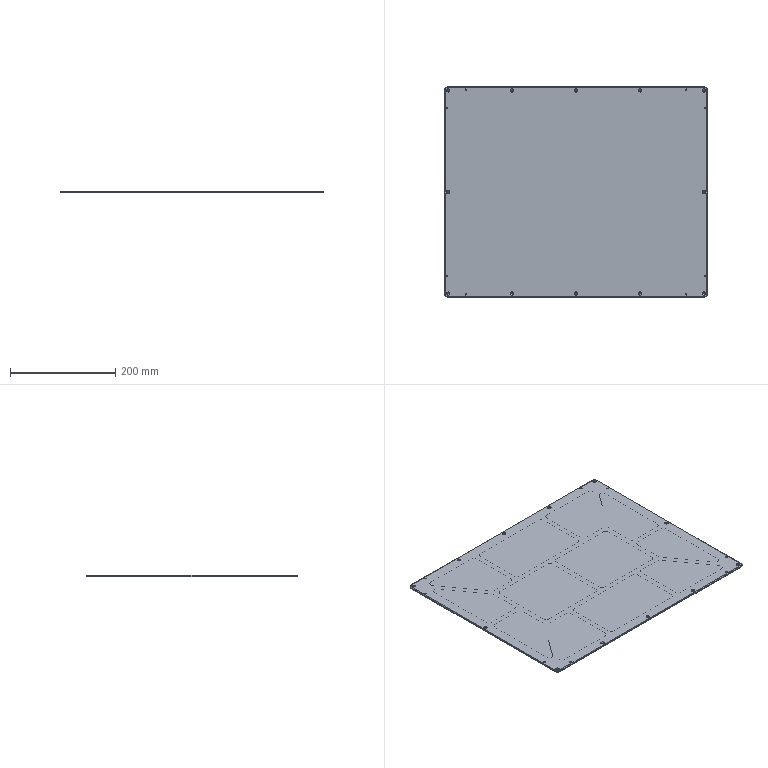NC program | Mastercam | posted with a generic post | part box 500 x 400 x 3 mm
Lines 1 to 214 of 11256:
%
:0001()
(MATERIAL - ALUMINUM MM - 2024)
(T9|10 FEM |H9|XY STOCK TO LEAVE - .15|Z STOCK TO LEAVE - .03)
(T10|10 FEM |H10|XY STOCK TO LEAVE - 0.|Z STOCK TO LEAVE - .03)
(T18|8 BNOS |H18)
(T5|4 CHM |H5)
(T8|8 FEM |H8|XY STOCK TO LEAVE - .1|Z STOCK TO LEAVE - 0.)
N100 G21
N102 G0 G17 G40 G80 G90 G94 G98
N104 G0 G28 G91 Z0.
N106 G0 G28 X0. Y0.
(10 FEM |TOOL - 9|DIA. OFF. - 9|LEN. - 9|TOOL DIA. - 10.)
N108 T9 M6
N110 G0 G54 G90 X253.177 Y-204.042 C0. B0. S10000 M3
N112 G43 H9 Z50.
N114 Z1.
N116 G1 Z0. F600.
N118 X252.57 Y-203.248 F5000.
N120 G3 X251.775 Y-202.855 I-.795 J-.607
N122 X251.168 Y-203.061 J-1.
N124 G1 X250.49 Y-203.537
N126 X249.776 Y-203.956 Z-.001
N128 X249.029 Y-204.316
N130 X248.256 Y-204.614
N132 X247.461 Y-204.847
N134 X246.65 Y-205.015 Z-.002
N136 X245.828 Y-205.116
N138 X245. Y-205.15
N140 X-245. Z-.136
N142 G2 X-255.15 Y-195. Z-.141 J10.15
N144 G1 Y195. Z-.247
N146 G2 X-245. Y205.15 Z-.252 I10.15
N148 G1 X245. Z-.386
N150 G2 X255.15 Y195. Z-.391 J-10.15
N152 G1 Y-195. Z-.497
N154 X255.115 Y-195.846
N156 X255.009 Y-196.686 Z-.498
N158 X254.834 Y-197.514
N160 X254.59 Y-198.324
N162 X254.28 Y-199.112
N164 X253.905 Y-199.871 Z-.499
N166 X253.468 Y-200.596
N168 X252.972 Y-201.282
N170 X252.421 Y-201.925
N172 X251.818 Y-202.519 Z-.5
N174 X251.168 Y-203.061
N176 X250.49 Y-203.537
N178 X249.776 Y-203.956
N180 X249.029 Y-204.316 Z-.501
N182 X248.256 Y-204.614
N184 X247.461 Y-204.847
N186 X246.65 Y-205.015
N188 X245.828 Y-205.116 Z-.502
N190 X245. Y-205.15
N192 X-245. Z-.636
N194 G2 X-255.15 Y-195. Z-.641 J10.15
N196 G1 Y195. Z-.747
N198 G2 X-245. Y205.15 Z-.752 I10.15
N200 G1 X245. Z-.886
N202 G2 X255.15 Y195. Z-.891 J-10.15
N204 G1 Y-195. Z-.997
N206 X255.115 Y-195.846
N208 X255.009 Y-196.686 Z-.998
N210 X254.834 Y-197.514
N212 X254.59 Y-198.324
N214 X254.28 Y-199.112
N216 X253.905 Y-199.871 Z-.999
N218 X253.468 Y-200.596
N220 X252.972 Y-201.282
N222 X252.421 Y-201.925
N224 X251.818 Y-202.519 Z-1.
N226 X251.168 Y-203.061
N228 X250.49 Y-203.537
N230 X249.776 Y-203.956
N232 X249.029 Y-204.316 Z-1.001
N234 X248.256 Y-204.614
N236 X247.461 Y-204.847
N238 X246.65 Y-205.015 Z-1.002
N240 X245.828 Y-205.116
N242 X245. Y-205.15
N244 X-245. Z-1.136
N246 G2 X-255.15 Y-195. Z-1.141 J10.15
N248 G1 Y195. Z-1.247
N250 G2 X-245. Y205.15 Z-1.252 I10.15
N252 G1 X245. Z-1.386
N254 G2 X255.15 Y195. Z-1.391 J-10.15
N256 G1 Y-195. Z-1.497
N258 X255.115 Y-195.846
N260 X255.009 Y-196.686 Z-1.498
N262 X254.834 Y-197.514
N264 X254.59 Y-198.324
N266 X254.28 Y-199.112
N268 X253.905 Y-199.871 Z-1.499
N270 X253.468 Y-200.596
N272 X252.972 Y-201.282
N274 X252.421 Y-201.925
N276 X251.818 Y-202.519 Z-1.5
N278 X251.168 Y-203.061
N280 X250.49 Y-203.537
N282 X249.776 Y-203.956
N284 X249.029 Y-204.316 Z-1.501
N286 X248.256 Y-204.614
N288 X247.461 Y-204.847
N290 X246.65 Y-205.015 Z-1.502
N292 X245.828 Y-205.116
N294 X245. Y-205.15
N296 X-245. Z-1.636
N298 G2 X-255.15 Y-195. Z-1.641 J10.15
N300 G1 Y195. Z-1.747
N302 G2 X-245. Y205.15 Z-1.752 I10.15
N304 G1 X245. Z-1.886
N306 G2 X255.15 Y195. Z-1.891 J-10.15
N308 G1 Y-195. Z-1.997
N310 X255.115 Y-195.846
N312 X255.009 Y-196.686 Z-1.998
N314 X254.834 Y-197.514
N316 X254.59 Y-198.324
N318 X254.28 Y-199.112
N320 X253.905 Y-199.871 Z-1.999
N322 X253.468 Y-200.596
N324 X252.972 Y-201.282
N326 X252.421 Y-201.925
N328 X251.818 Y-202.519 Z-2.
N330 X251.168 Y-203.061
N332 X250.49 Y-203.537
N334 X249.776 Y-203.956 Z-2.001
N336 X249.029 Y-204.316
N338 X248.256 Y-204.614
N340 X247.461 Y-204.847
N342 X246.65 Y-205.015 Z-2.002
N344 X245.828 Y-205.116
N346 X245. Y-205.15
N348 X-245. Z-2.136
N350 G2 X-255.15 Y-195. Z-2.141 J10.15
N352 G1 Y195. Z-2.247
N354 G2 X-245. Y205.15 Z-2.252 I10.15
N356 G1 X245. Z-2.386
N358 G2 X255.15 Y195. Z-2.391 J-10.15
N360 G1 Y-195. Z-2.497
N362 X255.115 Y-195.846
N364 X255.009 Y-196.686 Z-2.498
N366 X254.834 Y-197.514
N368 X254.59 Y-198.324
N370 X254.28 Y-199.112
N372 X253.905 Y-199.871 Z-2.499
N374 X253.468 Y-200.596
N376 X252.972 Y-201.282
N378 X252.421 Y-201.925
N380 X251.818 Y-202.519 Z-2.5
N382 X251.168 Y-203.061
N384 X250.49 Y-203.537
N386 X249.776 Y-203.956 Z-2.501
N388 X249.029 Y-204.316
N390 X248.256 Y-204.614
N392 X247.461 Y-204.847
N394 X246.65 Y-205.015 Z-2.502
N396 X245.828 Y-205.116
N398 X245. Y-205.15
N400 X-245. Z-2.636
N402 G2 X-255.15 Y-195. Z-2.641 J10.15
N404 G1 Y195. Z-2.747
N406 G2 X-245. Y205.15 Z-2.752 I10.15
N408 G1 X245. Z-2.886
N410 G2 X255.15 Y195. Z-2.891 J-10.15
N412 G1 Y-94.888 Z-2.97
N414 Y-195.
N416 G2 X251.168 Y-203.061 I-10.15
N418 X245. Y-205.15 I-6.168 J8.061
N420 G1 X-245.
N422 G2 X-255.15 Y-195. J10.15
N424 G1 Y195.
N426 G2 X-245. Y205.15 I10.15
N428 G1 X245.
N430 G2 X255.15 Y195. J-10.15
N432 G1 Y-95.388
N434 G3 X256.15 Y-96.388 I1.
N436 G1 X257.15
N438 G0 Z50.
N440 M5
N442 G0 G28 G91 Z0.
N444 G28
N446 M01
N448 G0 G17 G40 G80 G90 G94 G98
N450 G0 G28 G91 Z0.
(10 FEM |TOOL - 10|DIA. OFF. - 10|LEN. - 10|TOOL DIA. - 10.)
N452 T10 M6
N454 G0 G54 G90 X253.086 Y-203.923 C0. B0. S7000 M3
N456 G43 H10 Z50.
N458 Z1.
N460 G1 Z-2.97 F600.
N462 X252.479 Y-203.128 F1000.
N464 G3 X251.684 Y-202.735 I-.795 J-.608
N466 X251.077 Y-202.942 J-1.001
N468 G2 X245. Y-205. I-6.077 J7.942
N470 G1 X-245.
N472 G2 X-255. Y-195. J10.
N474 G1 Y195.
N476 G2 X-245. Y205. I10.
N478 G1 X245.
N480 G2 X255. Y195. J-10.
N482 G1 Y-195.
N484 G2 X251.077 Y-202.942 I-10.
N486 X250.672 Y-203.236 I-6.077 J7.942
N488 G3 X250.24 Y-204.059 I.567 J-.823
N490 X250.416 Y-204.627 I.999
N492 G1 X250.983 Y-205.45
N494 G0 Z50.
N496 M5
N498 G0 G28 G91 Z0.
N500 G28
N502 M01
N504 G0 G17 G40 G80 G90 G94 G98
N506 G0 G28 G91 Z0.